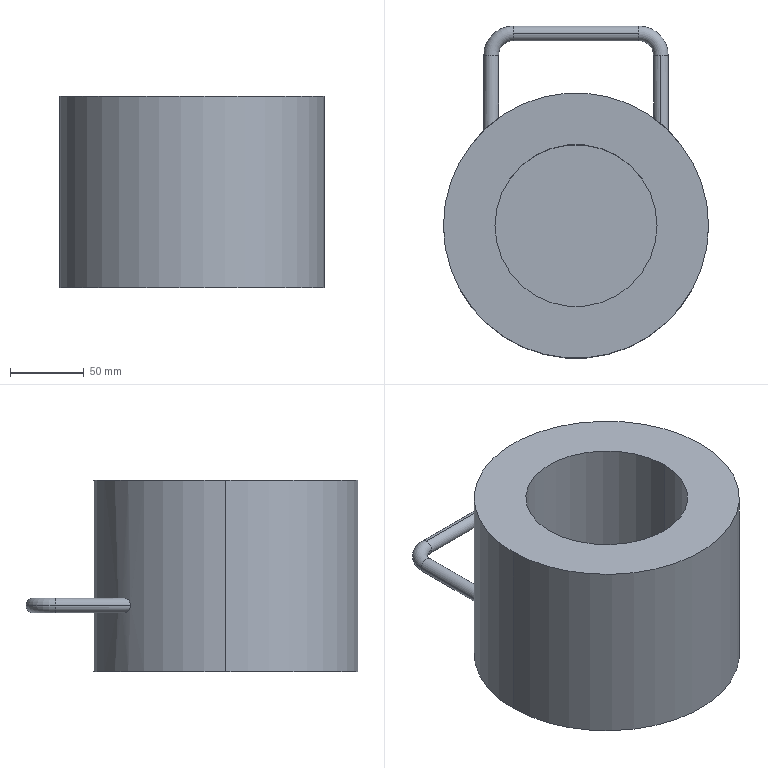Part | SolidWorks | features Extrusion 1, ICE 1, Sweep 1 | 1 solid | 17 faces | box 180 x 225.589 x 130 mm | volume 2375464 mm3 | cylinder 10 | torus 4 | plane 3 | commonest cylinder face diameters 10 x6 110 x2 180 x2
STEP:
#1=CARTESIAN_POINT('',(-42.6,130.589,50.));
#2=VERTEX_POINT('',#1);
#3=CARTESIAN_POINT('',(-42.6,135.589,45.));
#4=VERTEX_POINT('',#3);
#5=CARTESIAN_POINT('',(-42.6,130.589,45.));
#6=DIRECTION('',(-1.,0.,0.));
#7=DIRECTION('',(0.,0.,1.));
#8=AXIS2_PLACEMENT_3D('',#5,#6,#7);
#9=CIRCLE('',#8,5.);
#10=EDGE_CURVE('',#2,#4,#9,.T.);
#11=ORIENTED_EDGE('',*,*,#10,.T.);
#12=CARTESIAN_POINT('',(-62.6,115.589,45.));
#13=VERTEX_POINT('',#12);
#14=CARTESIAN_POINT('',(-42.6,115.589,45.));
#15=DIRECTION('',(0.,0.,1.));
#16=DIRECTION('',(1.,0.,0.));
#17=AXIS2_PLACEMENT_3D('',#14,#15,#16);
#18=CIRCLE('',#17,20.);
#19=EDGE_CURVE('',#4,#13,#18,.T.);
#20=ORIENTED_EDGE('',*,*,#19,.T.);
#21=CARTESIAN_POINT('',(-52.6,115.589,45.));
#22=VERTEX_POINT('',#21);
#23=CARTESIAN_POINT('',(-57.6,115.589,45.));
#24=DIRECTION('',(0.,-1.,0.));
#25=DIRECTION('',(0.,0.,1.));
#26=AXIS2_PLACEMENT_3D('',#23,#24,#25);
#27=CIRCLE('',#26,5.);
#28=EDGE_CURVE('',#22,#13,#27,.T.);
#29=ORIENTED_EDGE('',*,*,#28,.F.);
#30=CARTESIAN_POINT('',(-42.6,125.589,45.));
#31=VERTEX_POINT('',#30);
#32=CARTESIAN_POINT('',(-42.6,115.589,45.));
#33=DIRECTION('',(0.,0.,1.));
#34=DIRECTION('',(1.,0.,0.));
#35=AXIS2_PLACEMENT_3D('',#32,#33,#34);
#36=CIRCLE('',#35,10.);
#37=EDGE_CURVE('',#31,#22,#36,.T.);
#38=ORIENTED_EDGE('',*,*,#37,.F.);
#39=CARTESIAN_POINT('',(-42.6,130.589,45.));
#40=DIRECTION('',(-1.,0.,0.));
#41=DIRECTION('',(0.,0.,1.));
#42=AXIS2_PLACEMENT_3D('',#39,#40,#41);
#43=CIRCLE('',#42,5.);
#44=EDGE_CURVE('',#31,#2,#43,.T.);
#45=ORIENTED_EDGE('',*,*,#44,.T.);
#46=EDGE_LOOP('',(#11,#20,#29,#38,#45));
#47=FACE_OUTER_BOUND('',#46,.T.);
#48=CARTESIAN_POINT('',(-42.6,115.589,45.));
#49=DIRECTION('',(0.,0.,1.));
#50=DIRECTION('',(1.,0.,0.));
#51=AXIS2_PLACEMENT_3D('',#48,#49,#50);
#52=TOROIDAL_SURFACE('',#51,15.,5.);
#53=ADVANCED_FACE('',(#47),#52,.T.);
#54=CARTESIAN_POINT('',(57.6,115.589,50.));
#55=VERTEX_POINT('',#54);
#56=CARTESIAN_POINT('',(62.6,115.589,45.));
#57=VERTEX_POINT('',#56);
#58=CARTESIAN_POINT('',(57.6,115.589,45.));
#59=DIRECTION('',(0.,1.,0.));
#60=DIRECTION('',(0.,0.,1.));
#61=AXIS2_PLACEMENT_3D('',#58,#59,#60);
#62=CIRCLE('',#61,5.);
#63=EDGE_CURVE('',#55,#57,#62,.T.);
#64=ORIENTED_EDGE('',*,*,#63,.T.);
#65=CARTESIAN_POINT('',(42.6,135.589,45.));
#66=VERTEX_POINT('',#65);
#67=CARTESIAN_POINT('',(42.6,115.589,45.));
#68=DIRECTION('',(0.,0.,1.));
#69=DIRECTION('',(1.,0.,0.));
#70=AXIS2_PLACEMENT_3D('',#67,#68,#69);
#71=CIRCLE('',#70,20.);
#72=EDGE_CURVE('',#57,#66,#71,.T.);
#73=ORIENTED_EDGE('',*,*,#72,.T.);
#74=CARTESIAN_POINT('',(42.6,130.589,50.));
#75=VERTEX_POINT('',#74);
#76=CARTESIAN_POINT('',(42.6,130.589,45.));
#77=DIRECTION('',(-1.,0.,0.));
#78=DIRECTION('',(0.,0.,1.));
#79=AXIS2_PLACEMENT_3D('',#76,#77,#78);
#80=CIRCLE('',#79,5.);
#81=EDGE_CURVE('',#75,#66,#80,.T.);
#82=ORIENTED_EDGE('',*,*,#81,.F.);
#83=CARTESIAN_POINT('',(42.6,125.589,45.));
#84=VERTEX_POINT('',#83);
#85=CARTESIAN_POINT('',(42.6,130.589,45.));
#86=DIRECTION('',(-1.,0.,0.));
#87=DIRECTION('',(0.,0.,1.));
#88=AXIS2_PLACEMENT_3D('',#85,#86,#87);
#89=CIRCLE('',#88,5.);
#90=EDGE_CURVE('',#84,#75,#89,.T.);
#91=ORIENTED_EDGE('',*,*,#90,.F.);
#92=CARTESIAN_POINT('',(52.6,115.589,45.));
#93=VERTEX_POINT('',#92);
#94=CARTESIAN_POINT('',(42.6,115.589,45.));
#95=DIRECTION('',(0.,0.,1.));
#96=DIRECTION('',(1.,0.,0.));
#97=AXIS2_PLACEMENT_3D('',#94,#95,#96);
#98=CIRCLE('',#97,10.);
#99=EDGE_CURVE('',#93,#84,#98,.T.);
#100=ORIENTED_EDGE('',*,*,#99,.F.);
#101=CARTESIAN_POINT('',(57.6,115.589,45.));
#102=DIRECTION('',(0.,1.,0.));
#103=DIRECTION('',(0.,0.,1.));
#104=AXIS2_PLACEMENT_3D('',#101,#102,#103);
#105=CIRCLE('',#104,5.);
#106=EDGE_CURVE('',#93,#55,#105,.T.);
#107=ORIENTED_EDGE('',*,*,#106,.T.);
#108=EDGE_LOOP('',(#64,#73,#82,#91,#100,#107));
#109=FACE_OUTER_BOUND('',#108,.T.);
#110=CARTESIAN_POINT('',(42.6,115.589,45.));
#111=DIRECTION('',(0.,0.,1.));
#112=DIRECTION('',(1.,0.,0.));
#113=AXIS2_PLACEMENT_3D('',#110,#111,#112);
#114=TOROIDAL_SURFACE('',#113,15.,5.);
#115=ADVANCED_FACE('',(#109),#114,.T.);
#116=ORIENTED_EDGE('',*,*,#81,.T.);
#117=CARTESIAN_POINT('',(42.6,130.589,40.));
#118=VERTEX_POINT('',#117);
#119=CARTESIAN_POINT('',(42.6,130.589,45.));
#120=DIRECTION('',(-1.,0.,0.));
#121=DIRECTION('',(0.,0.,1.));
#122=AXIS2_PLACEMENT_3D('',#119,#120,#121);
#123=CIRCLE('',#122,5.);
#124=EDGE_CURVE('',#66,#118,#123,.T.);
#125=ORIENTED_EDGE('',*,*,#124,.T.);
#126=CARTESIAN_POINT('',(-42.6,130.589,40.));
#127=VERTEX_POINT('',#126);
#128=CARTESIAN_POINT('',(42.6,130.589,40.));
#129=DIRECTION('',(-1.,0.,0.));
#130=VECTOR('',#129,1000.);
#131=LINE('',#128,#130);
#132=EDGE_CURVE('',#118,#127,#131,.T.);
#133=ORIENTED_EDGE('',*,*,#132,.T.);
#134=CARTESIAN_POINT('',(-42.6,130.589,45.));
#135=DIRECTION('',(-1.,0.,0.));
#136=DIRECTION('',(0.,0.,1.));
#137=AXIS2_PLACEMENT_3D('',#134,#135,#136);
#138=CIRCLE('',#137,5.);
#139=EDGE_CURVE('',#4,#127,#138,.T.);
#140=ORIENTED_EDGE('',*,*,#139,.F.);
#141=ORIENTED_EDGE('',*,*,#10,.F.);
#142=CARTESIAN_POINT('',(42.6,130.589,50.));
#143=DIRECTION('',(-1.,0.,0.));
#144=VECTOR('',#143,1000.);
#145=LINE('',#142,#144);
#146=EDGE_CURVE('',#75,#2,#145,.T.);
#147=ORIENTED_EDGE('',*,*,#146,.F.);
#148=EDGE_LOOP('',(#116,#125,#133,#140,#141,#147));
#149=FACE_OUTER_BOUND('',#148,.T.);
#150=CARTESIAN_POINT('',(42.6,130.589,45.));
#151=DIRECTION('',(-1.,0.,0.));
#152=DIRECTION('',(0.,0.,1.));
#153=AXIS2_PLACEMENT_3D('',#150,#151,#152);
#154=CYLINDRICAL_SURFACE('',#153,5.);
#155=ADVANCED_FACE('',(#149),#154,.T.);
#156=ORIENTED_EDGE('',*,*,#28,.T.);
#157=CARTESIAN_POINT('',(-62.6,64.663,45.));
#158=VERTEX_POINT('',#157);
#159=CARTESIAN_POINT('',(-62.6,115.589,45.));
#160=DIRECTION('',(0.,-1.,0.));
#161=VECTOR('',#160,1000.);
#162=LINE('',#159,#161);
#163=EDGE_CURVE('',#13,#158,#162,.T.);
#164=ORIENTED_EDGE('',*,*,#163,.T.);
#165=CARTESIAN_POINT('',(-52.6,73.029,45.));
#166=VERTEX_POINT('',#165);
#167=CARTESIAN_POINT('',(-52.6,73.029,45.));
#168=CARTESIAN_POINT('',(-52.6,73.029,45.383));
#169=CARTESIAN_POINT('',(-52.643,72.998,45.757));
#170=CARTESIAN_POINT('',(-52.769,72.907,46.303));
#171=CARTESIAN_POINT('',(-52.822,72.869,46.484));
#172=CARTESIAN_POINT('',(-52.944,72.78,46.833));
#173=CARTESIAN_POINT('',(-53.014,72.729,47.001));
#174=CARTESIAN_POINT('',(-53.248,72.558,47.488));
#175=CARTESIAN_POINT('',(-53.439,72.418,47.793));
#176=CARTESIAN_POINT('',(-53.861,72.104,48.338));
#177=CARTESIAN_POINT('',(-54.095,71.929,48.581));
#178=CARTESIAN_POINT('',(-54.597,71.549,49.011));
#179=CARTESIAN_POINT('',(-54.86,71.348,49.194));
#180=CARTESIAN_POINT('',(-55.406,70.925,49.504));
#181=CARTESIAN_POINT('',(-55.69,70.702,49.631));
#182=CARTESIAN_POINT('',(-56.262,70.247,49.827));
#183=CARTESIAN_POINT('',(-56.551,70.015,49.898));
#184=CARTESIAN_POINT('',(-57.134,69.54,49.987));
#185=CARTESIAN_POINT('',(-57.429,69.297,50.005));
#186=CARTESIAN_POINT('',(-58.009,68.812,49.992));
#187=CARTESIAN_POINT('',(-58.295,68.57,49.96));
#188=CARTESIAN_POINT('',(-58.861,68.084,49.847));
#189=CARTESIAN_POINT('',(-59.143,67.84,49.765));
#190=CARTESIAN_POINT('',(-59.962,67.12,49.446));
#191=CARTESIAN_POINT('',(-60.47,66.661,49.142));
#192=CARTESIAN_POINT('',(-61.053,66.125,48.62));
#193=CARTESIAN_POINT('',(-61.167,66.02,48.507));
#194=CARTESIAN_POINT('',(-61.385,65.817,48.271));
#195=CARTESIAN_POINT('',(-61.489,65.72,48.146));
#196=CARTESIAN_POINT('',(-61.688,65.533,47.884));
#197=CARTESIAN_POINT('',(-61.782,65.445,47.746));
#198=CARTESIAN_POINT('',(-61.959,65.277,47.455));
#199=CARTESIAN_POINT('',(-62.043,65.197,47.301));
#200=CARTESIAN_POINT('',(-62.269,64.982,46.823));
#201=CARTESIAN_POINT('',(-62.39,64.866,46.484));
#202=CARTESIAN_POINT('',(-62.557,64.704,45.753));
#203=CARTESIAN_POINT('',(-62.6,64.663,45.379));
#204=CARTESIAN_POINT('',(-62.6,64.663,45.));
#205=B_SPLINE_CURVE_WITH_KNOTS('',3,(#167,#168,#169,#170,#171,#172,#173,#174,#175,#176,#177,#178,#179,#180,#181,#182,#183,#184,#185,#186,#187,#188,#189,#190,#191,#192,#193,#194,#195,#196,#197,#198,#199,#200,#201,#202,#203,#204),.UNSPECIFIED.,.F.,.F.,(4,2,2,2,2,2,2,2,2,2,2,2,2,2,2,2,2,2,4),(0.,0.001131,0.001697,0.002262,0.003394,0.004525,0.005656,0.006787,0.007918,0.009049,0.01018,0.01131,0.01357,0.01414,0.01471,0.01527,0.01584,0.01697,0.0181),.UNSPECIFIED.);
#206=EDGE_CURVE('',#166,#158,#205,.T.);
#207=ORIENTED_EDGE('',*,*,#206,.F.);
#208=CARTESIAN_POINT('',(-52.6,115.589,45.));
#209=DIRECTION('',(0.,-1.,0.));
#210=VECTOR('',#209,1000.);
#211=LINE('',#208,#210);
#212=EDGE_CURVE('',#22,#166,#211,.T.);
#213=ORIENTED_EDGE('',*,*,#212,.F.);
#214=EDGE_LOOP('',(#156,#164,#207,#213));
#215=FACE_OUTER_BOUND('',#214,.T.);
#216=CARTESIAN_POINT('',(-57.6,115.589,45.));
#217=DIRECTION('',(0.,-1.,0.));
#218=DIRECTION('',(1.,0.,0.));
#219=AXIS2_PLACEMENT_3D('',#216,#217,#218);
#220=CYLINDRICAL_SURFACE('',#219,5.);
#221=ADVANCED_FACE('',(#215),#220,.T.);
#222=CARTESIAN_POINT('',(57.6,69.154,40.));
#223=VERTEX_POINT('',#222);
#224=CARTESIAN_POINT('',(57.6,69.154,50.));
#225=VERTEX_POINT('',#224);
#226=CARTESIAN_POINT('',(57.6,69.154,40.));
#227=CARTESIAN_POINT('',(57.895,68.908,40.));
#228=CARTESIAN_POINT('',(58.192,68.658,40.026));
#229=CARTESIAN_POINT('',(58.769,68.164,40.13));
#230=CARTESIAN_POINT('',(59.052,67.919,40.206));
#231=CARTESIAN_POINT('',(59.606,67.433,40.411));
#232=CARTESIAN_POINT('',(59.879,67.191,40.539));
#233=CARTESIAN_POINT('',(60.405,66.719,40.849));
#234=CARTESIAN_POINT('',(60.655,66.491,41.029));
#235=CARTESIAN_POINT('',(61.01,66.165,41.34));
#236=CARTESIAN_POINT('',(61.126,66.058,41.451));
#237=CARTESIAN_POINT('',(61.349,65.851,41.687));
#238=CARTESIAN_POINT('',(61.457,65.75,41.814));
#239=CARTESIAN_POINT('',(61.764,65.462,42.211));
#240=CARTESIAN_POINT('',(61.946,65.29,42.502));
#241=CARTESIAN_POINT('',(62.179,65.067,42.984));
#242=CARTESIAN_POINT('',(62.25,65.,43.153));
#243=CARTESIAN_POINT('',(62.373,64.882,43.498));
#244=CARTESIAN_POINT('',(62.425,64.831,43.676));
#245=CARTESIAN_POINT('',(62.511,64.749,44.042));
#246=CARTESIAN_POINT('',(62.544,64.716,44.233));
#247=CARTESIAN_POINT('',(62.589,64.673,44.614));
#248=CARTESIAN_POINT('',(62.6,64.663,44.805));
#249=CARTESIAN_POINT('',(62.6,64.662,45.38));
#250=CARTESIAN_POINT('',(62.555,64.707,45.77));
#251=CARTESIAN_POINT('',(62.384,64.871,46.502));
#252=CARTESIAN_POINT('',(62.257,64.993,46.854));
#253=CARTESIAN_POINT('',(61.948,65.287,47.494));
#254=CARTESIAN_POINT('',(61.765,65.461,47.786));
#255=CARTESIAN_POINT('',(61.355,65.846,48.319));
#256=CARTESIAN_POINT('',(61.132,66.053,48.553));
#257=CARTESIAN_POINT('',(60.658,66.488,48.968));
#258=CARTESIAN_POINT('',(60.405,66.718,49.15));
#259=CARTESIAN_POINT('',(59.88,67.19,49.46));
#260=CARTESIAN_POINT('',(59.61,67.43,49.588));
#261=CARTESIAN_POINT('',(59.057,67.915,49.792));
#262=CARTESIAN_POINT('',(58.774,68.16,49.869));
#263=CARTESIAN_POINT('',(58.193,68.657,49.973));
#264=CARTESIAN_POINT('',(57.897,68.907,50.));
#265=CARTESIAN_POINT('',(57.6,69.154,50.));
#266=B_SPLINE_CURVE_WITH_KNOTS('',3,(#226,#227,#228,#229,#230,#231,#232,#233,#234,#235,#236,#237,#238,#239,#240,#241,#242,#243,#244,#245,#246,#247,#248,#249,#250,#251,#252,#253,#254,#255,#256,#257,#258,#259,#260,#261,#262,#263,#264,#265),.UNSPECIFIED.,.F.,.F.,(4,2,2,2,2,2,2,2,2,2,2,2,2,2,2,2,2,2,2,4),(0.01776,0.0189,0.02004,0.02119,0.02233,0.02291,0.02348,0.02462,0.02519,0.02577,0.02634,0.02691,0.02806,0.0292,0.03034,0.03149,0.03263,0.03378,0.03492,0.03607),.UNSPECIFIED.);
#267=EDGE_CURVE('',#223,#225,#266,.T.);
#268=ORIENTED_EDGE('',*,*,#267,.F.);
#269=CARTESIAN_POINT('',(57.6,115.589,40.));
#270=VERTEX_POINT('',#269);
#271=CARTESIAN_POINT('',(57.6,56.789,40.));
#272=DIRECTION('',(0.,1.,0.));
#273=VECTOR('',#272,1000.);
#274=LINE('',#271,#273);
#275=EDGE_CURVE('',#223,#270,#274,.T.);
#276=ORIENTED_EDGE('',*,*,#275,.T.);
#277=CARTESIAN_POINT('',(57.6,115.589,45.));
#278=DIRECTION('',(0.,1.,0.));
#279=DIRECTION('',(0.,0.,1.));
#280=AXIS2_PLACEMENT_3D('',#277,#278,#279);
#281=CIRCLE('',#280,5.);
#282=EDGE_CURVE('',#57,#270,#281,.T.);
#283=ORIENTED_EDGE('',*,*,#282,.F.);
#284=ORIENTED_EDGE('',*,*,#63,.F.);
#285=CARTESIAN_POINT('',(57.6,56.789,50.));
#286=DIRECTION('',(0.,1.,0.));
#287=VECTOR('',#286,1000.);
#288=LINE('',#285,#287);
#289=EDGE_CURVE('',#225,#55,#288,.T.);
#290=ORIENTED_EDGE('',*,*,#289,.F.);
#291=EDGE_LOOP('',(#268,#276,#283,#284,#290));
#292=FACE_OUTER_BOUND('',#291,.T.);
#293=CARTESIAN_POINT('',(57.6,56.789,45.));
#294=DIRECTION('',(0.,1.,0.));
#295=DIRECTION('',(0.,0.,1.));
#296=AXIS2_PLACEMENT_3D('',#293,#294,#295);
#297=CYLINDRICAL_SURFACE('',#296,5.);
#298=ADVANCED_FACE('',(#292),#297,.T.);
#299=CARTESIAN_POINT('',(-55.,0.,30.));
#300=VERTEX_POINT('',#299);
#301=CARTESIAN_POINT('',(55.,0.,30.));
#302=VERTEX_POINT('',#301);
#303=CARTESIAN_POINT('',(0.,0.,30.));
#304=DIRECTION('',(0.,0.,1.));
#305=DIRECTION('',(1.,0.,0.));
#306=AXIS2_PLACEMENT_3D('',#303,#304,#305);
#307=CIRCLE('',#306,55.);
#308=EDGE_CURVE('',#300,#302,#307,.T.);
#309=ORIENTED_EDGE('',*,*,#308,.F.);
#310=CARTESIAN_POINT('',(-55.,0.,130.));
#311=VERTEX_POINT('',#310);
#312=CARTESIAN_POINT('',(-55.,0.,30.));
#313=DIRECTION('',(0.,0.,1.));
#314=VECTOR('',#313,1000.);
#315=LINE('',#312,#314);
#316=EDGE_CURVE('',#300,#311,#315,.T.);
#317=ORIENTED_EDGE('',*,*,#316,.T.);
#318=CARTESIAN_POINT('',(55.,0.,130.));
#319=VERTEX_POINT('',#318);
#320=CARTESIAN_POINT('',(0.,0.,130.));
#321=DIRECTION('',(0.,0.,1.));
#322=DIRECTION('',(1.,0.,0.));
#323=AXIS2_PLACEMENT_3D('',#320,#321,#322);
#324=CIRCLE('',#323,55.);
#325=EDGE_CURVE('',#311,#319,#324,.T.);
#326=ORIENTED_EDGE('',*,*,#325,.T.);
#327=CARTESIAN_POINT('',(55.,0.,30.));
#328=DIRECTION('',(0.,0.,1.));
#329=VECTOR('',#328,1000.);
#330=LINE('',#327,#329);
#331=EDGE_CURVE('',#302,#319,#330,.T.);
#332=ORIENTED_EDGE('',*,*,#331,.F.);
#333=EDGE_LOOP('',(#309,#317,#326,#332));
#334=FACE_OUTER_BOUND('',#333,.T.);
#335=CARTESIAN_POINT('',(0.,0.,30.));
#336=DIRECTION('',(0.,0.,1.));
#337=DIRECTION('',(1.,0.,0.));
#338=AXIS2_PLACEMENT_3D('',#335,#336,#337);
#339=CYLINDRICAL_SURFACE('',#338,55.);
#340=ADVANCED_FACE('',(#334),#339,.F.);
#341=CARTESIAN_POINT('',(57.6,69.154,50.));
#342=CARTESIAN_POINT('',(57.025,69.633,50.));
#343=CARTESIAN_POINT('',(56.455,70.095,49.904));
#344=CARTESIAN_POINT('',(55.612,70.763,49.598));
#345=CARTESIAN_POINT('',(55.334,70.981,49.468));
#346=CARTESIAN_POINT('',(54.802,71.392,49.155));
#347=CARTESIAN_POINT('',(54.546,71.588,48.972));
#348=CARTESIAN_POINT('',(54.18,71.865,48.651));
#349=CARTESIAN_POINT('',(54.061,71.955,48.536));
#350=CARTESIAN_POINT('',(53.834,72.124,48.293));
#351=CARTESIAN_POINT('',(53.726,72.205,48.165));
#352=CARTESIAN_POINT('',(53.521,72.357,47.896));
#353=CARTESIAN_POINT('',(53.424,72.429,47.755));
#354=CARTESIAN_POINT('',(53.242,72.562,47.457));
#355=CARTESIAN_POINT('',(53.157,72.625,47.3));
#356=CARTESIAN_POINT('',(52.929,72.791,46.818));
#357=CARTESIAN_POINT('',(52.81,72.878,46.479));
#358=CARTESIAN_POINT('',(52.686,72.967,45.942));
#359=CARTESIAN_POINT('',(52.654,72.99,45.756));
#360=CARTESIAN_POINT('',(52.611,73.021,45.386));
#361=CARTESIAN_POINT('',(52.59,73.036,45.016));
#362=CARTESIAN_POINT('',(52.609,73.022,44.645));
#363=CARTESIAN_POINT('',(52.65,72.993,44.273));
#364=CARTESIAN_POINT('',(52.68,72.971,44.088));
#365=CARTESIAN_POINT('',(52.761,72.913,43.728));
#366=CARTESIAN_POINT('',(52.811,72.877,43.553));
#367=CARTESIAN_POINT('',(52.928,72.792,43.209));
#368=CARTESIAN_POINT('',(52.997,72.742,43.04));
#369=CARTESIAN_POINT('',(53.225,72.575,42.554));
#370=CARTESIAN_POINT('',(53.406,72.442,42.257));
#371=CARTESIAN_POINT('',(53.819,72.136,41.71));
#372=CARTESIAN_POINT('',(54.048,71.965,41.467));
#373=CARTESIAN_POINT('',(54.534,71.597,41.037));
#374=CARTESIAN_POINT('',(54.794,71.398,40.85));
#375=CARTESIAN_POINT('',(55.329,70.984,40.535));
#376=CARTESIAN_POINT('',(55.604,70.769,40.406));
#377=CARTESIAN_POINT('',(56.167,70.323,40.2));
#378=CARTESIAN_POINT('',(56.455,70.093,40.124));
#379=CARTESIAN_POINT('',(57.027,69.628,40.024));
#380=CARTESIAN_POINT('',(57.314,69.392,40.));
#381=CARTESIAN_POINT('',(57.6,69.154,40.));
#382=B_SPLINE_CURVE_WITH_KNOTS('',3,(#341,#342,#343,#344,#345,#346,#347,#348,#349,#350,#351,#352,#353,#354,#355,#356,#357,#358,#359,#360,#361,#362,#363,#364,#365,#366,#367,#368,#369,#370,#371,#372,#373,#374,#375,#376,#377,#378,#379,#380,#381),.UNSPECIFIED.,.F.,.F.,(4,2,2,2,2,2,2,2,2,2,1,2,2,2,2,2,2,2,2,2,4),(0.,0.002219,0.003329,0.004439,0.004994,0.005549,0.006103,0.006658,0.007768,0.008323,0.008878,0.009433,0.009987,0.01054,0.0111,0.01221,0.01332,0.01443,0.01554,0.01665,0.01776),.UNSPECIFIED.);
#383=EDGE_CURVE('',#225,#223,#382,.T.);
#384=ORIENTED_EDGE('',*,*,#383,.T.);
#385=ORIENTED_EDGE('',*,*,#267,.T.);
#386=EDGE_LOOP('',(#384,#385));
#387=FACE_BOUND('',#386,.T.);
#388=ORIENTED_EDGE('',*,*,#206,.T.);
#389=CARTESIAN_POINT('',(-62.6,64.663,45.));
#390=CARTESIAN_POINT('',(-62.6,64.663,44.811));
#391=CARTESIAN_POINT('',(-62.589,64.673,44.618));
#392=CARTESIAN_POINT('',(-62.546,64.715,44.243));
#393=CARTESIAN_POINT('',(-62.514,64.746,44.059));
#394=CARTESIAN_POINT('',(-62.431,64.826,43.698));
#395=CARTESIAN_POINT('',(-62.379,64.876,43.519));
#396=CARTESIAN_POINT('',(-62.259,64.991,43.176));
#397=CARTESIAN_POINT('',(-62.191,65.056,43.011));
#398=CARTESIAN_POINT('',(-61.965,65.272,42.536));
#399=CARTESIAN_POINT('',(-61.783,65.444,42.242));
#400=CARTESIAN_POINT('',(-61.386,65.816,41.718));
#401=CARTESIAN_POINT('',(-61.169,66.018,41.484));
#402=CARTESIAN_POINT('',(-60.702,66.448,41.066));
#403=CARTESIAN_POINT('',(-60.454,66.674,40.884));
#404=CARTESIAN_POINT('',(-59.944,67.133,40.574));
#405=CARTESIAN_POINT('',(-59.68,67.368,40.444));
#406=CARTESIAN_POINT('',(-59.135,67.847,40.232));
#407=CARTESIAN_POINT('',(-58.852,68.092,40.151));
#408=CARTESIAN_POINT('',(-58.285,68.578,40.039));
#409=CARTESIAN_POINT('',(-57.999,68.821,40.008));
#410=CARTESIAN_POINT('',(-57.42,69.304,39.995));
#411=CARTESIAN_POINT('',(-57.126,69.547,40.014));
#412=CARTESIAN_POINT('',(-56.543,70.022,40.104));
#413=CARTESIAN_POINT('',(-56.255,70.253,40.175));
#414=CARTESIAN_POINT('',(-55.689,70.703,40.37));
#415=CARTESIAN_POINT('',(-55.41,70.922,40.494));
#416=CARTESIAN_POINT('',(-54.999,71.24,40.727));
#417=CARTESIAN_POINT('',(-54.863,71.344,40.812));
#418=CARTESIAN_POINT('',(-54.6,71.546,40.997));
#419=CARTESIAN_POINT('',(-54.472,71.644,41.096));
#420=CARTESIAN_POINT('',(-54.099,71.926,41.415));
#421=CARTESIAN_POINT('',(-53.865,72.102,41.658));
#422=CARTESIAN_POINT('',(-53.438,72.419,42.207));
#423=CARTESIAN_POINT('',(-53.251,72.556,42.506));
#424=CARTESIAN_POINT('',(-53.016,72.728,42.995));
#425=CARTESIAN_POINT('',(-52.945,72.779,43.166));
#426=CARTESIAN_POINT('',(-52.822,72.869,43.515));
#427=CARTESIAN_POINT('',(-52.77,72.906,43.693));
#428=CARTESIAN_POINT('',(-52.686,72.967,44.056));
#429=CARTESIAN_POINT('',(-52.654,72.99,44.24));
#430=CARTESIAN_POINT('',(-52.611,73.021,44.616));
#431=CARTESIAN_POINT('',(-52.6,73.029,44.809));
#432=CARTESIAN_POINT('',(-52.6,73.029,45.));
#433=B_SPLINE_CURVE_WITH_KNOTS('',3,(#389,#390,#391,#392,#393,#394,#395,#396,#397,#398,#399,#400,#401,#402,#403,#404,#405,#406,#407,#408,#409,#410,#411,#412,#413,#414,#415,#416,#417,#418,#419,#420,#421,#422,#423,#424,#425,#426,#427,#428,#429,#430,#431,#432),.UNSPECIFIED.,.F.,.F.,(4,2,2,2,2,2,2,2,2,2,2,2,2,2,2,2,2,2,2,2,2,4),(0.0181,0.01866,0.01923,0.01979,0.02036,0.02149,0.02262,0.02375,0.02488,0.02601,0.02714,0.02827,0.0294,0.03053,0.03109,0.03166,0.03278,0.03391,0.03448,0.03504,0.03561,0.03617),.UNSPECIFIED.);
#434=EDGE_CURVE('',#158,#166,#433,.T.);
#435=ORIENTED_EDGE('',*,*,#434,.T.);
#436=EDGE_LOOP('',(#388,#435));
#437=FACE_BOUND('',#436,.T.);
#438=CARTESIAN_POINT('',(90.,0.,130.));
#439=VERTEX_POINT('',#438);
#440=CARTESIAN_POINT('',(-90.,0.,130.));
#441=VERTEX_POINT('',#440);
#442=CARTESIAN_POINT('',(0.,0.,130.));
#443=DIRECTION('',(0.,0.,1.));
#444=DIRECTION('',(1.,0.,0.));
#445=AXIS2_PLACEMENT_3D('',#442,#443,#444);
#446=CIRCLE('',#445,90.);
#447=EDGE_CURVE('',#439,#441,#446,.T.);
#448=ORIENTED_EDGE('',*,*,#447,.F.);
#449=CARTESIAN_POINT('',(90.,0.,0.));
#450=VERTEX_POINT('',#449);
#451=CARTESIAN_POINT('',(90.,0.,130.));
#452=DIRECTION('',(0.,0.,-1.));
#453=VECTOR('',#452,1000.);
#454=LINE('',#451,#453);
#455=EDGE_CURVE('',#439,#450,#454,.T.);
#456=ORIENTED_EDGE('',*,*,#455,.T.);
#457=CARTESIAN_POINT('',(-90.,0.,0.));
#458=VERTEX_POINT('',#457);
#459=CARTESIAN_POINT('',(0.,0.,0.));
#460=DIRECTION('',(0.,0.,1.));
#461=DIRECTION('',(1.,0.,0.));
#462=AXIS2_PLACEMENT_3D('',#459,#460,#461);
#463=CIRCLE('',#462,90.);
#464=EDGE_CURVE('',#450,#458,#463,.T.);
#465=ORIENTED_EDGE('',*,*,#464,.T.);
#466=CARTESIAN_POINT('',(-90.,0.,130.));
#467=DIRECTION('',(0.,0.,-1.));
#468=VECTOR('',#467,1000.);
#469=LINE('',#466,#468);
#470=EDGE_CURVE('',#441,#458,#469,.T.);
#471=ORIENTED_EDGE('',*,*,#470,.F.);
#472=EDGE_LOOP('',(#448,#456,#465,#471));
#473=FACE_OUTER_BOUND('',#472,.T.);
#474=CARTESIAN_POINT('',(0.,0.,130.));
#475=DIRECTION('',(0.,0.,-1.));
#476=DIRECTION('',(-1.,0.,0.));
#477=AXIS2_PLACEMENT_3D('',#474,#475,#476);
#478=CYLINDRICAL_SURFACE('',#477,90.);
#479=ADVANCED_FACE('',(#387,#437,#473),#478,.T.);
#480=ORIENTED_EDGE('',*,*,#455,.F.);
#481=CARTESIAN_POINT('',(0.,0.,130.));
#482=DIRECTION('',(0.,0.,1.));
#483=DIRECTION('',(1.,0.,0.));
#484=AXIS2_PLACEMENT_3D('',#481,#482,#483);
#485=CIRCLE('',#484,90.);
#486=EDGE_CURVE('',#441,#439,#485,.T.);
#487=ORIENTED_EDGE('',*,*,#486,.F.);
#488=ORIENTED_EDGE('',*,*,#470,.T.);
#489=CARTESIAN_POINT('',(0.,0.,0.));
#490=DIRECTION('',(0.,0.,1.));
#491=DIRECTION('',(1.,0.,0.));
#492=AXIS2_PLACEMENT_3D('',#489,#490,#491);
#493=CIRCLE('',#492,90.);
#494=EDGE_CURVE('',#458,#450,#493,.T.);
#495=ORIENTED_EDGE('',*,*,#494,.T.);
#496=EDGE_LOOP('',(#480,#487,#488,#495));
#497=FACE_OUTER_BOUND('',#496,.T.);
#498=CARTESIAN_POINT('',(0.,0.,130.));
#499=DIRECTION('',(0.,0.,-1.));
#500=DIRECTION('',(-1.,0.,0.));
#501=AXIS2_PLACEMENT_3D('',#498,#499,#500);
#502=CYLINDRICAL_SURFACE('',#501,90.);
#503=ADVANCED_FACE('',(#497),#502,.T.);
#504=CARTESIAN_POINT('',(0.,0.,130.));
#505=DIRECTION('',(0.,0.,1.));
#506=DIRECTION('',(1.,0.,0.));
#507=AXIS2_PLACEMENT_3D('',#504,#505,#506);
#508=CIRCLE('',#507,55.);
#509=EDGE_CURVE('',#319,#311,#508,.T.);
#510=ORIENTED_EDGE('',*,*,#509,.F.);
#511=ORIENTED_EDGE('',*,*,#325,.F.);
#512=EDGE_LOOP('',(#510,#511));
#513=FACE_BOUND('',#512,.T.);
#514=ORIENTED_EDGE('',*,*,#486,.T.);
#515=ORIENTED_EDGE('',*,*,#447,.T.);
#516=EDGE_LOOP('',(#514,#515));
#517=FACE_OUTER_BOUND('',#516,.T.);
#518=CARTESIAN_POINT('',(0.,0.,130.));
#519=DIRECTION('',(0.,0.,1.));
#520=DIRECTION('',(1.,0.,0.));
#521=AXIS2_PLACEMENT_3D('',#518,#519,#520);
#522=PLANE('',#521);
#523=ADVANCED_FACE('',(#513,#517),#522,.T.);
#524=ORIENTED_EDGE('',*,*,#494,.F.);
#525=ORIENTED_EDGE('',*,*,#464,.F.);
#526=EDGE_LOOP('',(#524,#525));
#527=FACE_OUTER_BOUND('',#526,.T.);
#528=CARTESIAN_POINT('',(0.,0.,0.));
#529=DIRECTION('',(0.,0.,1.));
#530=DIRECTION('',(1.,0.,0.));
#531=AXIS2_PLACEMENT_3D('',#528,#529,#530);
#532=PLANE('',#531);
#533=ADVANCED_FACE('',(#527),#532,.F.);
#534=ORIENTED_EDGE('',*,*,#316,.F.);
#535=CARTESIAN_POINT('',(0.,0.,30.));
#536=DIRECTION('',(0.,0.,1.));
#537=DIRECTION('',(1.,0.,0.));
#538=AXIS2_PLACEMENT_3D('',#535,#536,#537);
#539=CIRCLE('',#538,55.);
#540=EDGE_CURVE('',#302,#300,#539,.T.);
#541=ORIENTED_EDGE('',*,*,#540,.F.);
#542=ORIENTED_EDGE('',*,*,#331,.T.);
#543=ORIENTED_EDGE('',*,*,#509,.T.);
#544=EDGE_LOOP('',(#534,#541,#542,#543));
#545=FACE_OUTER_BOUND('',#544,.T.);
#546=CARTESIAN_POINT('',(0.,0.,30.));
#547=DIRECTION('',(0.,0.,1.));
#548=DIRECTION('',(1.,0.,0.));
#549=AXIS2_PLACEMENT_3D('',#546,#547,#548);
#550=CYLINDRICAL_SURFACE('',#549,55.);
#551=ADVANCED_FACE('',(#545),#550,.F.);
#552=ORIENTED_EDGE('',*,*,#540,.T.);
#553=ORIENTED_EDGE('',*,*,#308,.T.);
#554=EDGE_LOOP('',(#552,#553));
#555=FACE_OUTER_BOUND('',#554,.T.);
#556=CARTESIAN_POINT('',(0.,0.,30.));
#557=DIRECTION('',(0.,0.,1.));
#558=DIRECTION('',(1.,0.,0.));
#559=AXIS2_PLACEMENT_3D('',#556,#557,#558);
#560=PLANE('',#559);
#561=ADVANCED_FACE('',(#555),#560,.T.);
#562=ORIENTED_EDGE('',*,*,#275,.F.);
#563=ORIENTED_EDGE('',*,*,#383,.F.);
#564=ORIENTED_EDGE('',*,*,#289,.T.);
#565=ORIENTED_EDGE('',*,*,#106,.F.);
#566=CARTESIAN_POINT('',(57.6,115.589,45.));
#567=DIRECTION('',(0.,1.,0.));
#568=DIRECTION('',(0.,0.,1.));
#569=AXIS2_PLACEMENT_3D('',#566,#567,#568);
#570=CIRCLE('',#569,5.);
#571=EDGE_CURVE('',#270,#93,#570,.T.);
#572=ORIENTED_EDGE('',*,*,#571,.F.);
#573=EDGE_LOOP('',(#562,#563,#564,#565,#572));
#574=FACE_OUTER_BOUND('',#573,.T.);
#575=CARTESIAN_POINT('',(57.6,56.789,45.));
#576=DIRECTION('',(0.,1.,0.));
#577=DIRECTION('',(0.,0.,1.));
#578=AXIS2_PLACEMENT_3D('',#575,#576,#577);
#579=CYLINDRICAL_SURFACE('',#578,5.);
#580=ADVANCED_FACE('',(#574),#579,.T.);
#581=ORIENTED_EDGE('',*,*,#163,.F.);
#582=CARTESIAN_POINT('',(-57.6,115.589,45.));
#583=DIRECTION('',(0.,-1.,0.));
#584=DIRECTION('',(0.,0.,1.));
#585=AXIS2_PLACEMENT_3D('',#582,#583,#584);
#586=CIRCLE('',#585,5.);
#587=EDGE_CURVE('',#13,#22,#586,.T.);
#588=ORIENTED_EDGE('',*,*,#587,.T.);
#589=ORIENTED_EDGE('',*,*,#212,.T.);
#590=ORIENTED_EDGE('',*,*,#434,.F.);
#591=EDGE_LOOP('',(#581,#588,#589,#590));
#592=FACE_OUTER_BOUND('',#591,.T.);
#593=CARTESIAN_POINT('',(-57.6,115.589,45.));
#594=DIRECTION('',(0.,-1.,0.));
#595=DIRECTION('',(1.,0.,0.));
#596=AXIS2_PLACEMENT_3D('',#593,#594,#595);
#597=CYLINDRICAL_SURFACE('',#596,5.);
#598=ADVANCED_FACE('',(#592),#597,.T.);
#599=ORIENTED_EDGE('',*,*,#19,.F.);
#600=ORIENTED_EDGE('',*,*,#139,.T.);
#601=CARTESIAN_POINT('',(-42.6,130.589,45.));
#602=DIRECTION('',(-1.,0.,0.));
#603=DIRECTION('',(0.,0.,1.));
#604=AXIS2_PLACEMENT_3D('',#601,#602,#603);
#605=CIRCLE('',#604,5.);
#606=EDGE_CURVE('',#127,#31,#605,.T.);
#607=ORIENTED_EDGE('',*,*,#606,.T.);
#608=ORIENTED_EDGE('',*,*,#37,.T.);
#609=ORIENTED_EDGE('',*,*,#587,.F.);
#610=EDGE_LOOP('',(#599,#600,#607,#608,#609));
#611=FACE_OUTER_BOUND('',#610,.T.);
#612=CARTESIAN_POINT('',(-42.6,115.589,45.));
#613=DIRECTION('',(0.,0.,1.));
#614=DIRECTION('',(1.,0.,0.));
#615=AXIS2_PLACEMENT_3D('',#612,#613,#614);
#616=TOROIDAL_SURFACE('',#615,15.,5.);
#617=ADVANCED_FACE('',(#611),#616,.T.);
#618=ORIENTED_EDGE('',*,*,#132,.F.);
#619=CARTESIAN_POINT('',(42.6,130.589,45.));
#620=DIRECTION('',(-1.,0.,0.));
#621=DIRECTION('',(0.,0.,1.));
#622=AXIS2_PLACEMENT_3D('',#619,#620,#621);
#623=CIRCLE('',#622,5.);
#624=EDGE_CURVE('',#118,#84,#623,.T.);
#625=ORIENTED_EDGE('',*,*,#624,.T.);
#626=ORIENTED_EDGE('',*,*,#90,.T.);
#627=ORIENTED_EDGE('',*,*,#146,.T.);
#628=ORIENTED_EDGE('',*,*,#44,.F.);
#629=ORIENTED_EDGE('',*,*,#606,.F.);
#630=EDGE_LOOP('',(#618,#625,#626,#627,#628,#629));
#631=FACE_OUTER_BOUND('',#630,.T.);
#632=CARTESIAN_POINT('',(42.6,130.589,45.));
#633=DIRECTION('',(-1.,0.,0.));
#634=DIRECTION('',(0.,0.,1.));
#635=AXIS2_PLACEMENT_3D('',#632,#633,#634);
#636=CYLINDRICAL_SURFACE('',#635,5.);
#637=ADVANCED_FACE('',(#631),#636,.T.);
#638=ORIENTED_EDGE('',*,*,#72,.F.);
#639=ORIENTED_EDGE('',*,*,#282,.T.);
#640=ORIENTED_EDGE('',*,*,#571,.T.);
#641=ORIENTED_EDGE('',*,*,#99,.T.);
#642=ORIENTED_EDGE('',*,*,#624,.F.);
#643=ORIENTED_EDGE('',*,*,#124,.F.);
#644=EDGE_LOOP('',(#638,#639,#640,#641,#642,#643));
#645=FACE_OUTER_BOUND('',#644,.T.);
#646=CARTESIAN_POINT('',(42.6,115.589,45.));
#647=DIRECTION('',(0.,0.,1.));
#648=DIRECTION('',(1.,0.,0.));
#649=AXIS2_PLACEMENT_3D('',#646,#647,#648);
#650=TOROIDAL_SURFACE('',#649,15.,5.);
#651=ADVANCED_FACE('',(#645),#650,.T.);
#652=CLOSED_SHELL('',(#53,#115,#155,#221,#298,#340,#479,#503,#523,#533,#551,#561,#580,#598,#617,#637,#651));
#653=MANIFOLD_SOLID_BREP('',#652);
#654=CARTESIAN_POINT('',(0.,0.,0.));
#655=DIRECTION('',(0.,0.,1.));
#656=DIRECTION('',(1.,0.,0.));
#657=AXIS2_PLACEMENT_3D('',#654,#655,#656);
#658=(LENGTH_UNIT()NAMED_UNIT(*)SI_UNIT(.MILLI.,.METRE.));
#659=UNCERTAINTY_MEASURE_WITH_UNIT(LENGTH_MEASURE(0.00001),#658,'','');
#660=(NAMED_UNIT(*)PLANE_ANGLE_UNIT()SI_UNIT($,.RADIAN.));
#661=(NAMED_UNIT(*)SI_UNIT($,.STERADIAN.)SOLID_ANGLE_UNIT());
#662=(GEOMETRIC_REPRESENTATION_CONTEXT(3)GLOBAL_UNCERTAINTY_ASSIGNED_CONTEXT((#659))GLOBAL_UNIT_ASSIGNED_CONTEXT((#658,#660,#661))REPRESENTATION_CONTEXT('',''));
#663=ADVANCED_BREP_SHAPE_REPRESENTATION('',(#653,#657),#662);